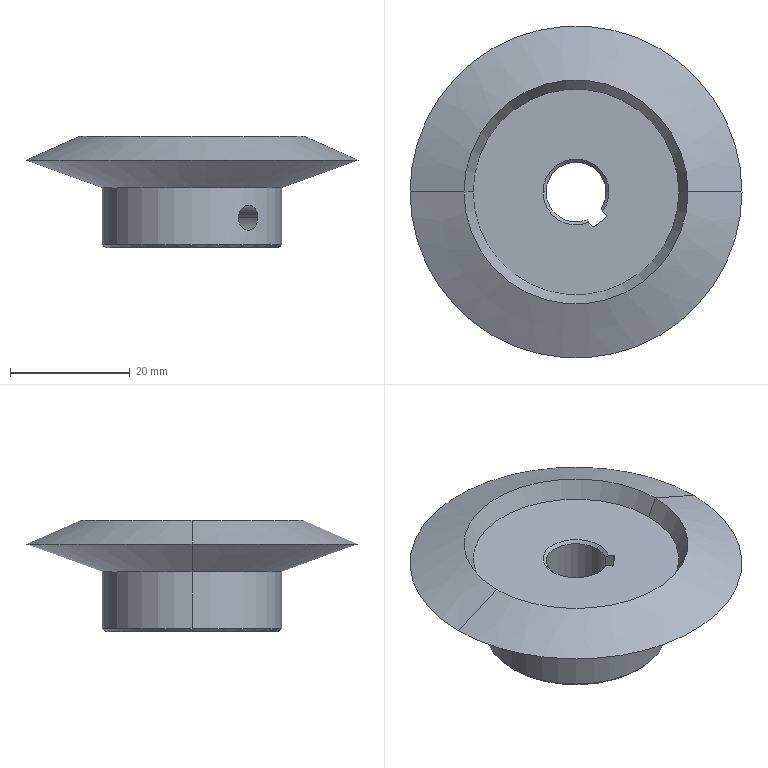Part | SolidWorks | features BaseBody 1 | 1 solid | 33 faces | box 55.34 x 55.34 x 18.54 mm | volume 16079 mm3 | cone 14 | cylinder 11 | plane 8 | commonest cylinder face diameters 0.4 x4 10 x3 4.2 x2 30 x2
STEP:
#1=CARTESIAN_POINT('',(-119.453,1729.544,-1197.43));
#2=VERTEX_POINT('',#1);
#3=CARTESIAN_POINT('',(-149.453,1729.544,-1197.43));
#4=VERTEX_POINT('',#3);
#5=CARTESIAN_POINT('',(-134.453,1729.544,-1197.43));
#6=DIRECTION('',(0.,0.,1.));
#7=DIRECTION('',(-0.7769,-0.6296,0.));
#8=AXIS2_PLACEMENT_3D('',#5,#6,#7);
#9=CIRCLE('',#8,15.);
#10=EDGE_CURVE('',#2,#4,#9,.T.);
#11=ORIENTED_EDGE('',*,*,#10,.T.);
#12=CARTESIAN_POINT('',(-162.123,1729.544,-1192.84));
#13=VERTEX_POINT('',#12);
#14=CARTESIAN_POINT('',(-162.123,1729.544,-1192.84));
#15=DIRECTION('',(-0.9402,0.,0.3406));
#16=VECTOR('',#15,1000.);
#17=LINE('',#14,#16);
#18=EDGE_CURVE('',#4,#13,#17,.T.);
#19=ORIENTED_EDGE('',*,*,#18,.T.);
#20=CARTESIAN_POINT('',(-106.783,1729.544,-1192.84));
#21=VERTEX_POINT('',#20);
#22=CARTESIAN_POINT('',(-134.453,1729.544,-1192.84));
#23=DIRECTION('',(0.,0.,-1.));
#24=DIRECTION('',(-0.7769,-0.6296,0.));
#25=AXIS2_PLACEMENT_3D('',#22,#23,#24);
#26=CIRCLE('',#25,27.67);
#27=EDGE_CURVE('',#13,#21,#26,.T.);
#28=ORIENTED_EDGE('',*,*,#27,.T.);
#29=CARTESIAN_POINT('',(-106.783,1729.544,-1192.84));
#30=DIRECTION('',(0.9402,0.,0.3406));
#31=VECTOR('',#30,1000.);
#32=LINE('',#29,#31);
#33=EDGE_CURVE('',#2,#21,#32,.T.);
#34=ORIENTED_EDGE('',*,*,#33,.F.);
#35=EDGE_LOOP('',(#11,#19,#28,#34));
#36=FACE_OUTER_BOUND('',#35,.T.);
#37=CARTESIAN_POINT('',(-134.453,1729.544,-1192.84));
#38=DIRECTION('',(0.,0.,1.));
#39=DIRECTION('',(1.,0.,0.));
#40=AXIS2_PLACEMENT_3D('',#37,#38,#39);
#41=CONICAL_SURFACE('',#40,27.67,1.223);
#42=ADVANCED_FACE('',(#36),#41,.T.);
#43=CARTESIAN_POINT('',(-153.134,1729.544,-1188.89));
#44=VERTEX_POINT('',#43);
#45=CARTESIAN_POINT('',(-115.773,1729.544,-1188.89));
#46=VERTEX_POINT('',#45);
#47=CARTESIAN_POINT('',(-134.453,1729.544,-1188.89));
#48=DIRECTION('',(0.,0.,-1.));
#49=DIRECTION('',(0.7769,0.6296,0.));
#50=AXIS2_PLACEMENT_3D('',#47,#48,#49);
#51=CIRCLE('',#50,18.68);
#52=EDGE_CURVE('',#44,#46,#51,.T.);
#53=ORIENTED_EDGE('',*,*,#52,.T.);
#54=CARTESIAN_POINT('',(-106.783,1729.544,-1192.84));
#55=DIRECTION('',(0.9155,0.,-0.4023));
#56=VECTOR('',#55,1000.);
#57=LINE('',#54,#56);
#58=EDGE_CURVE('',#46,#21,#57,.T.);
#59=ORIENTED_EDGE('',*,*,#58,.T.);
#60=ORIENTED_EDGE('',*,*,#27,.F.);
#61=CARTESIAN_POINT('',(-162.123,1729.544,-1192.84));
#62=DIRECTION('',(-0.9155,0.,-0.4023));
#63=VECTOR('',#62,1000.);
#64=LINE('',#61,#63);
#65=EDGE_CURVE('',#44,#13,#64,.T.);
#66=ORIENTED_EDGE('',*,*,#65,.F.);
#67=EDGE_LOOP('',(#53,#59,#60,#66));
#68=FACE_OUTER_BOUND('',#67,.T.);
#69=CARTESIAN_POINT('',(-134.453,1729.544,-1192.84));
#70=DIRECTION('',(0.,0.,-1.));
#71=DIRECTION('',(-1.,0.,0.));
#72=AXIS2_PLACEMENT_3D('',#69,#70,#71);
#73=CONICAL_SURFACE('',#72,27.67,1.157);
#74=ADVANCED_FACE('',(#68),#73,.T.);
#75=CARTESIAN_POINT('',(-119.453,1729.544,-1206.93));
#76=VERTEX_POINT('',#75);
#77=CARTESIAN_POINT('',(-149.453,1729.544,-1206.93));
#78=VERTEX_POINT('',#77);
#79=CARTESIAN_POINT('',(-134.453,1729.544,-1206.93));
#80=DIRECTION('',(0.,0.,1.));
#81=DIRECTION('',(1.,0.,0.));
#82=AXIS2_PLACEMENT_3D('',#79,#80,#81);
#83=CIRCLE('',#82,15.);
#84=EDGE_CURVE('',#76,#78,#83,.T.);
#85=ORIENTED_EDGE('',*,*,#84,.T.);
#86=CARTESIAN_POINT('',(-149.453,1729.544,-1180.68));
#87=DIRECTION('',(0.,0.,1.));
#88=VECTOR('',#87,1000.);
#89=LINE('',#86,#88);
#90=EDGE_CURVE('',#78,#4,#89,.T.);
#91=ORIENTED_EDGE('',*,*,#90,.T.);
#92=ORIENTED_EDGE('',*,*,#10,.F.);
#93=CARTESIAN_POINT('',(-119.453,1729.544,-1180.68));
#94=DIRECTION('',(0.,0.,1.));
#95=VECTOR('',#94,1000.);
#96=LINE('',#93,#95);
#97=EDGE_CURVE('',#76,#2,#96,.T.);
#98=ORIENTED_EDGE('',*,*,#97,.F.);
#99=EDGE_LOOP('',(#85,#91,#92,#98));
#100=FACE_OUTER_BOUND('',#99,.T.);
#101=CARTESIAN_POINT('',(-134.453,1729.544,-1180.68));
#102=DIRECTION('',(0.,0.,1.));
#103=DIRECTION('',(1.,0.,0.));
#104=AXIS2_PLACEMENT_3D('',#101,#102,#103);
#105=CYLINDRICAL_SURFACE('',#104,15.);
#106=ADVANCED_FACE('',(#100),#105,.T.);
#107=CARTESIAN_POINT('',(-151.603,1729.544,-1191.93));
#108=VERTEX_POINT('',#107);
#109=CARTESIAN_POINT('',(-117.303,1729.544,-1191.93));
#110=VERTEX_POINT('',#109);
#111=CARTESIAN_POINT('',(-134.453,1729.544,-1191.93));
#112=DIRECTION('',(0.,0.,1.));
#113=DIRECTION('',(1.,0.,0.));
#114=AXIS2_PLACEMENT_3D('',#111,#112,#113);
#115=CIRCLE('',#114,17.15);
#116=EDGE_CURVE('',#108,#110,#115,.T.);
#117=ORIENTED_EDGE('',*,*,#116,.F.);
#118=CARTESIAN_POINT('',(-153.134,1729.544,-1188.89));
#119=DIRECTION('',(-0.4496,0.,0.8932));
#120=VECTOR('',#119,1000.);
#121=LINE('',#118,#120);
#122=EDGE_CURVE('',#108,#44,#121,.T.);
#123=ORIENTED_EDGE('',*,*,#122,.T.);
#124=CARTESIAN_POINT('',(-134.453,1729.544,-1188.89));
#125=DIRECTION('',(0.,0.,-1.));
#126=DIRECTION('',(0.7769,0.6296,0.));
#127=AXIS2_PLACEMENT_3D('',#124,#125,#126);
#128=CIRCLE('',#127,18.68);
#129=EDGE_CURVE('',#46,#44,#128,.T.);
#130=ORIENTED_EDGE('',*,*,#129,.F.);
#131=CARTESIAN_POINT('',(-115.773,1729.544,-1188.89));
#132=DIRECTION('',(0.4496,0.,0.8932));
#133=VECTOR('',#132,1000.);
#134=LINE('',#131,#133);
#135=EDGE_CURVE('',#110,#46,#134,.T.);
#136=ORIENTED_EDGE('',*,*,#135,.F.);
#137=EDGE_LOOP('',(#117,#123,#130,#136));
#138=FACE_OUTER_BOUND('',#137,.T.);
#139=CARTESIAN_POINT('',(-134.453,1729.544,-1188.89));
#140=DIRECTION('',(0.,0.,1.));
#141=DIRECTION('',(1.,0.,0.));
#142=AXIS2_PLACEMENT_3D('',#139,#140,#141);
#143=CONICAL_SURFACE('',#142,18.68,0.4663);
#144=ADVANCED_FACE('',(#138),#143,.F.);
#145=CARTESIAN_POINT('',(-133.228,1724.696,-1202.43));
#146=VERTEX_POINT('',#145);
#147=CARTESIAN_POINT('',(-132.616,1724.894,-1203.9));
#148=VERTEX_POINT('',#147);
#149=CARTESIAN_POINT('',(-133.228,1724.696,-1202.43));
#150=CARTESIAN_POINT('',(-133.228,1724.696,-1202.569));
#151=CARTESIAN_POINT('',(-133.214,1724.7,-1202.704));
#152=CARTESIAN_POINT('',(-133.158,1724.715,-1202.971));
#153=CARTESIAN_POINT('',(-133.115,1724.726,-1203.104));
#154=CARTESIAN_POINT('',(-132.954,1724.773,-1203.479));
#155=CARTESIAN_POINT('',(-132.8,1724.821,-1203.707));
#156=CARTESIAN_POINT('',(-132.616,1724.894,-1203.9));
#157=B_SPLINE_CURVE_WITH_KNOTS('',3,(#149,#150,#151,#152,#153,#154,#155,#156),.UNSPECIFIED.,.F.,.F.,(4,2,2,4),(0.001639,0.002049,0.002458,0.003277),.UNSPECIFIED.);
#158=EDGE_CURVE('',#146,#148,#157,.T.);
#159=ORIENTED_EDGE('',*,*,#158,.F.);
#160=CARTESIAN_POINT('',(-126.734,1716.683,-1202.43));
#161=VERTEX_POINT('',#160);
#162=CARTESIAN_POINT('',(-126.641,1716.568,-1202.43));
#163=DIRECTION('',(0.6296,-0.7769,0.));
#164=VECTOR('',#163,1000.);
#165=LINE('',#162,#164);
#166=EDGE_CURVE('',#146,#161,#165,.T.);
#167=ORIENTED_EDGE('',*,*,#166,.T.);
#168=CARTESIAN_POINT('',(-123.471,1719.327,-1202.43));
#169=VERTEX_POINT('',#168);
#170=CARTESIAN_POINT('',(-123.471,1719.327,-1202.43));
#171=CARTESIAN_POINT('',(-123.471,1719.327,-1202.569));
#172=CARTESIAN_POINT('',(-123.48,1719.317,-1202.705));
#173=CARTESIAN_POINT('',(-123.517,1719.278,-1202.974));
#174=CARTESIAN_POINT('',(-123.545,1719.248,-1203.107));
#175=CARTESIAN_POINT('',(-123.618,1719.171,-1203.362));
#176=CARTESIAN_POINT('',(-123.663,1719.124,-1203.482));
#177=CARTESIAN_POINT('',(-123.771,1719.014,-1203.71));
#178=CARTESIAN_POINT('',(-123.833,1718.951,-1203.818));
#179=CARTESIAN_POINT('',(-124.04,1718.746,-1204.108));
#180=CARTESIAN_POINT('',(-124.21,1718.583,-1204.265));
#181=CARTESIAN_POINT('',(-124.586,1718.244,-1204.474));
#182=CARTESIAN_POINT('',(-124.795,1718.064,-1204.53));
#183=CARTESIAN_POINT('',(-125.115,1717.805,-1204.53));
#184=CARTESIAN_POINT('',(-125.224,1717.719,-1204.516));
#185=CARTESIAN_POINT('',(-125.438,1717.555,-1204.463));
#186=CARTESIAN_POINT('',(-125.543,1717.476,-1204.423));
#187=CARTESIAN_POINT('',(-125.75,1717.327,-1204.318));
#188=CARTESIAN_POINT('',(-125.85,1717.256,-1204.252));
#189=CARTESIAN_POINT('',(-126.038,1717.126,-1204.101));
#190=CARTESIAN_POINT('',(-126.127,1717.067,-1204.014));
#191=CARTESIAN_POINT('',(-126.291,1716.959,-1203.818));
#192=CARTESIAN_POINT('',(-126.365,1716.912,-1203.712));
#193=CARTESIAN_POINT('',(-126.494,1716.83,-1203.485));
#194=CARTESIAN_POINT('',(-126.55,1716.795,-1203.362));
#195=CARTESIAN_POINT('',(-126.641,1716.739,-1203.108));
#196=CARTESIAN_POINT('',(-126.675,1716.718,-1202.977));
#197=CARTESIAN_POINT('',(-126.722,1716.69,-1202.708));
#198=CARTESIAN_POINT('',(-126.734,1716.683,-1202.569));
#199=CARTESIAN_POINT('',(-126.734,1716.683,-1202.43));
#200=B_SPLINE_CURVE_WITH_KNOTS('',3,(#170,#171,#172,#173,#174,#175,#176,#177,#178,#179,#180,#181,#182,#183,#184,#185,#186,#187,#188,#189,#190,#191,#192,#193,#194,#195,#196,#197,#198,#199),.UNSPECIFIED.,.F.,.F.,(4,2,2,2,2,2,2,2,2,2,2,2,2,2,4),(0.006572,0.006983,0.007394,0.007804,0.008215,0.009037,0.009858,0.01027,0.01068,0.01109,0.0115,0.01191,0.01232,0.01273,0.01314),.UNSPECIFIED.);
#201=EDGE_CURVE('',#169,#161,#200,.T.);
#202=ORIENTED_EDGE('',*,*,#201,.F.);
#203=CARTESIAN_POINT('',(-129.965,1727.341,-1202.43));
#204=VERTEX_POINT('',#203);
#205=CARTESIAN_POINT('',(-123.378,1719.212,-1202.43));
#206=DIRECTION('',(0.6296,-0.7769,0.));
#207=VECTOR('',#206,1000.);
#208=LINE('',#205,#207);
#209=EDGE_CURVE('',#204,#169,#208,.T.);
#210=ORIENTED_EDGE('',*,*,#209,.F.);
#211=CARTESIAN_POINT('',(-130.285,1726.783,-1203.9));
#212=VERTEX_POINT('',#211);
#213=CARTESIAN_POINT('',(-130.285,1726.783,-1203.9));
#214=CARTESIAN_POINT('',(-130.23,1726.865,-1203.803));
#215=CARTESIAN_POINT('',(-130.184,1726.941,-1203.699));
#216=CARTESIAN_POINT('',(-130.104,1727.077,-1203.476));
#217=CARTESIAN_POINT('',(-130.07,1727.137,-1203.355));
#218=CARTESIAN_POINT('',(-130.018,1727.236,-1203.104));
#219=CARTESIAN_POINT('',(-129.998,1727.275,-1202.975));
#220=CARTESIAN_POINT('',(-129.972,1727.327,-1202.707));
#221=CARTESIAN_POINT('',(-129.965,1727.341,-1202.569));
#222=CARTESIAN_POINT('',(-129.965,1727.341,-1202.43));
#223=B_SPLINE_CURVE_WITH_KNOTS('',3,(#213,#214,#215,#216,#217,#218,#219,#220,#221,#222),.UNSPECIFIED.,.F.,.F.,(4,2,2,2,4),(-0.001639,-0.001229,-0.0008193,-0.0004097,0.),.UNSPECIFIED.);
#224=EDGE_CURVE('',#212,#204,#223,.T.);
#225=ORIENTED_EDGE('',*,*,#224,.F.);
#226=CARTESIAN_POINT('',(-129.385,1725.671,-1203.9));
#227=VERTEX_POINT('',#226);
#228=CARTESIAN_POINT('',(-123.844,1718.835,-1203.9));
#229=DIRECTION('',(-0.6296,0.7769,0.));
#230=VECTOR('',#229,1000.);
#231=LINE('',#228,#230);
#232=EDGE_CURVE('',#227,#212,#231,.T.);
#233=ORIENTED_EDGE('',*,*,#232,.F.);
#234=CARTESIAN_POINT('',(-129.414,1725.39,-1204.079));
#235=VERTEX_POINT('',#234);
#236=CARTESIAN_POINT('',(-129.414,1725.39,-1204.079));
#237=CARTESIAN_POINT('',(-129.376,1725.421,-1204.041));
#238=CARTESIAN_POINT('',(-129.351,1725.463,-1204.001));
#239=CARTESIAN_POINT('',(-129.334,1725.562,-1203.931));
#240=CARTESIAN_POINT('',(-129.345,1725.623,-1203.9));
#241=CARTESIAN_POINT('',(-129.385,1725.671,-1203.9));
#242=B_SPLINE_CURVE_WITH_KNOTS('',3,(#236,#237,#238,#239,#240,#241),.UNSPECIFIED.,.F.,.F.,(4,2,4),(0.,0.0001833,0.0003667),.UNSPECIFIED.);
#243=EDGE_CURVE('',#235,#227,#242,.T.);
#244=ORIENTED_EDGE('',*,*,#243,.F.);
#245=CARTESIAN_POINT('',(-131.434,1723.753,-1204.079));
#246=VERTEX_POINT('',#245);
#247=CARTESIAN_POINT('',(-130.424,1724.572,-1202.43));
#248=DIRECTION('',(0.6296,-0.7769,0.));
#249=DIRECTION('',(0.7769,0.6296,0.));
#250=AXIS2_PLACEMENT_3D('',#247,#248,#249);
#251=CIRCLE('',#250,2.1);
#252=EDGE_CURVE('',#246,#235,#251,.T.);
#253=ORIENTED_EDGE('',*,*,#252,.F.);
#254=CARTESIAN_POINT('',(-131.715,1723.783,-1203.9));
#255=VERTEX_POINT('',#254);
#256=CARTESIAN_POINT('',(-131.715,1723.783,-1203.9));
#257=CARTESIAN_POINT('',(-131.676,1723.734,-1203.9));
#258=CARTESIAN_POINT('',(-131.619,1723.711,-1203.93));
#259=CARTESIAN_POINT('',(-131.518,1723.707,-1204.001));
#260=CARTESIAN_POINT('',(-131.472,1723.723,-1204.041));
#261=CARTESIAN_POINT('',(-131.434,1723.753,-1204.079));
#262=B_SPLINE_CURVE_WITH_KNOTS('',3,(#256,#257,#258,#259,#260,#261),.UNSPECIFIED.,.F.,.F.,(4,2,4),(0.,0.0001836,0.0003672),.UNSPECIFIED.);
#263=EDGE_CURVE('',#255,#246,#262,.T.);
#264=ORIENTED_EDGE('',*,*,#263,.F.);
#265=CARTESIAN_POINT('',(-126.175,1716.946,-1203.9));
#266=DIRECTION('',(0.6296,-0.7769,0.));
#267=VECTOR('',#266,1000.);
#268=LINE('',#265,#267);
#269=EDGE_CURVE('',#148,#255,#268,.T.);
#270=ORIENTED_EDGE('',*,*,#269,.F.);
#271=EDGE_LOOP('',(#159,#167,#202,#210,#225,#233,#244,#253,#264,#270));
#272=FACE_OUTER_BOUND('',#271,.T.);
#273=CARTESIAN_POINT('',(-125.01,1717.89,-1202.43));
#274=DIRECTION('',(0.6296,-0.7769,0.));
#275=DIRECTION('',(0.7769,0.6296,0.));
#276=AXIS2_PLACEMENT_3D('',#273,#274,#275);
#277=CYLINDRICAL_SURFACE('',#276,2.1);
#278=ADVANCED_FACE('',(#272),#277,.F.);
#279=CARTESIAN_POINT('',(-119.953,1729.544,-1207.43));
#280=VERTEX_POINT('',#279);
#281=CARTESIAN_POINT('',(-148.953,1729.544,-1207.43));
#282=VERTEX_POINT('',#281);
#283=CARTESIAN_POINT('',(-134.453,1729.544,-1207.43));
#284=DIRECTION('',(0.,0.,1.));
#285=DIRECTION('',(1.,0.,0.));
#286=AXIS2_PLACEMENT_3D('',#283,#284,#285);
#287=CIRCLE('',#286,14.5);
#288=EDGE_CURVE('',#280,#282,#287,.T.);
#289=ORIENTED_EDGE('',*,*,#288,.T.);
#290=CARTESIAN_POINT('',(-149.453,1729.544,-1206.93));
#291=DIRECTION('',(-0.7071,0.,0.7071));
#292=VECTOR('',#291,1000.);
#293=LINE('',#290,#292);
#294=EDGE_CURVE('',#282,#78,#293,.T.);
#295=ORIENTED_EDGE('',*,*,#294,.T.);
#296=ORIENTED_EDGE('',*,*,#84,.F.);
#297=CARTESIAN_POINT('',(-119.453,1729.544,-1206.93));
#298=DIRECTION('',(0.7071,0.,0.7071));
#299=VECTOR('',#298,1000.);
#300=LINE('',#297,#299);
#301=EDGE_CURVE('',#280,#76,#300,.T.);
#302=ORIENTED_EDGE('',*,*,#301,.F.);
#303=EDGE_LOOP('',(#289,#295,#296,#302));
#304=FACE_OUTER_BOUND('',#303,.T.);
#305=CARTESIAN_POINT('',(-134.453,1729.544,-1206.93));
#306=DIRECTION('',(0.,0.,1.));
#307=DIRECTION('',(1.,0.,0.));
#308=AXIS2_PLACEMENT_3D('',#305,#306,#307);
#309=CONICAL_SURFACE('',#308,15.,0.7854);
#310=ADVANCED_FACE('',(#304),#309,.T.);
#311=CARTESIAN_POINT('',(-139.453,1729.544,-1206.93));
#312=VERTEX_POINT('',#311);
#313=CARTESIAN_POINT('',(-132.616,1724.894,-1206.93));
#314=VERTEX_POINT('',#313);
#315=CARTESIAN_POINT('',(-134.453,1729.544,-1206.93));
#316=DIRECTION('',(0.,0.,1.));
#317=DIRECTION('',(1.,0.,0.));
#318=AXIS2_PLACEMENT_3D('',#315,#316,#317);
#319=CIRCLE('',#318,5.);
#320=EDGE_CURVE('',#312,#314,#319,.T.);
#321=ORIENTED_EDGE('',*,*,#320,.F.);
#322=CARTESIAN_POINT('',(-139.453,1729.544,-1192.43));
#323=VERTEX_POINT('',#322);
#324=CARTESIAN_POINT('',(-139.453,1729.544,-1180.68));
#325=DIRECTION('',(0.,0.,1.));
#326=VECTOR('',#325,1000.);
#327=LINE('',#324,#326);
#328=EDGE_CURVE('',#312,#323,#327,.T.);
#329=ORIENTED_EDGE('',*,*,#328,.T.);
#330=CARTESIAN_POINT('',(-132.616,1724.894,-1192.43));
#331=VERTEX_POINT('',#330);
#332=CARTESIAN_POINT('',(-134.453,1729.544,-1192.43));
#333=DIRECTION('',(0.,0.,-1.));
#334=DIRECTION('',(1.,0.,0.));
#335=AXIS2_PLACEMENT_3D('',#332,#333,#334);
#336=CIRCLE('',#335,5.);
#337=EDGE_CURVE('',#331,#323,#336,.T.);
#338=ORIENTED_EDGE('',*,*,#337,.F.);
#339=CARTESIAN_POINT('',(-132.616,1724.894,-1200.96));
#340=VERTEX_POINT('',#339);
#341=CARTESIAN_POINT('',(-132.616,1724.894,-1188.89));
#342=DIRECTION('',(0.,0.,-1.));
#343=VECTOR('',#342,1000.);
#344=LINE('',#341,#343);
#345=EDGE_CURVE('',#331,#340,#344,.T.);
#346=ORIENTED_EDGE('',*,*,#345,.T.);
#347=CARTESIAN_POINT('',(-132.616,1724.894,-1200.96));
#348=CARTESIAN_POINT('',(-132.708,1724.857,-1201.057));
#349=CARTESIAN_POINT('',(-132.792,1724.828,-1201.161));
#350=CARTESIAN_POINT('',(-132.941,1724.778,-1201.384));
#351=CARTESIAN_POINT('',(-133.007,1724.757,-1201.505));
#352=CARTESIAN_POINT('',(-133.115,1724.726,-1201.756));
#353=CARTESIAN_POINT('',(-133.157,1724.715,-1201.885));
#354=CARTESIAN_POINT('',(-133.213,1724.7,-1202.153));
#355=CARTESIAN_POINT('',(-133.228,1724.696,-1202.291));
#356=CARTESIAN_POINT('',(-133.228,1724.696,-1202.43));
#357=B_SPLINE_CURVE_WITH_KNOTS('',3,(#347,#348,#349,#350,#351,#352,#353,#354,#355,#356),.UNSPECIFIED.,.F.,.F.,(4,2,2,2,4),(0.,0.0004098,0.0008196,0.001229,0.001639),.UNSPECIFIED.);
#358=EDGE_CURVE('',#340,#146,#357,.T.);
#359=ORIENTED_EDGE('',*,*,#358,.T.);
#360=ORIENTED_EDGE('',*,*,#158,.T.);
#361=CARTESIAN_POINT('',(-132.616,1724.894,-1180.68));
#362=DIRECTION('',(0.,0.,1.));
#363=VECTOR('',#362,1000.);
#364=LINE('',#361,#363);
#365=EDGE_CURVE('',#314,#148,#364,.T.);
#366=ORIENTED_EDGE('',*,*,#365,.F.);
#367=EDGE_LOOP('',(#321,#329,#338,#346,#359,#360,#366));
#368=FACE_OUTER_BOUND('',#367,.T.);
#369=CARTESIAN_POINT('',(-134.453,1729.544,-1180.68));
#370=DIRECTION('',(0.,0.,1.));
#371=DIRECTION('',(1.,0.,0.));
#372=AXIS2_PLACEMENT_3D('',#369,#370,#371);
#373=CYLINDRICAL_SURFACE('',#372,5.);
#374=ADVANCED_FACE('',(#368),#373,.F.);
#375=ORIENTED_EDGE('',*,*,#328,.F.);
#376=CARTESIAN_POINT('',(-129.453,1729.544,-1206.93));
#377=VERTEX_POINT('',#376);
#378=CARTESIAN_POINT('',(-134.453,1729.544,-1206.93));
#379=DIRECTION('',(0.,0.,1.));
#380=DIRECTION('',(1.,0.,0.));
#381=AXIS2_PLACEMENT_3D('',#378,#379,#380);
#382=CIRCLE('',#381,5.);
#383=EDGE_CURVE('',#377,#312,#382,.T.);
#384=ORIENTED_EDGE('',*,*,#383,.F.);
#385=CARTESIAN_POINT('',(-129.453,1729.544,-1192.43));
#386=VERTEX_POINT('',#385);
#387=CARTESIAN_POINT('',(-129.453,1729.544,-1180.68));
#388=DIRECTION('',(0.,0.,1.));
#389=VECTOR('',#388,1000.);
#390=LINE('',#387,#389);
#391=EDGE_CURVE('',#377,#386,#390,.T.);
#392=ORIENTED_EDGE('',*,*,#391,.T.);
#393=CARTESIAN_POINT('',(-134.453,1729.544,-1192.43));
#394=DIRECTION('',(0.,0.,-1.));
#395=DIRECTION('',(1.,0.,0.));
#396=AXIS2_PLACEMENT_3D('',#393,#394,#395);
#397=CIRCLE('',#396,5.);
#398=EDGE_CURVE('',#323,#386,#397,.T.);
#399=ORIENTED_EDGE('',*,*,#398,.F.);
#400=EDGE_LOOP('',(#375,#384,#392,#399));
#401=FACE_OUTER_BOUND('',#400,.T.);
#402=CARTESIAN_POINT('',(-134.453,1729.544,-1180.68));
#403=DIRECTION('',(0.,0.,1.));
#404=DIRECTION('',(1.,0.,0.));
#405=AXIS2_PLACEMENT_3D('',#402,#403,#404);
#406=CYLINDRICAL_SURFACE('',#405,5.);
#407=ADVANCED_FACE('',(#401),#406,.F.);
#408=ORIENTED_EDGE('',*,*,#337,.T.);
#409=CARTESIAN_POINT('',(-139.953,1729.544,-1191.93));
#410=VERTEX_POINT('',#409);
#411=CARTESIAN_POINT('',(-139.953,1729.544,-1191.93));
#412=DIRECTION('',(-0.7071,0.,0.7071));
#413=VECTOR('',#412,1000.);
#414=LINE('',#411,#413);
#415=EDGE_CURVE('',#323,#410,#414,.T.);
#416=ORIENTED_EDGE('',*,*,#415,.T.);
#417=CARTESIAN_POINT('',(-132.287,1724.489,-1191.93));
#418=VERTEX_POINT('',#417);
#419=CARTESIAN_POINT('',(-134.453,1729.544,-1191.93));
#420=DIRECTION('',(0.,0.,1.));
#421=DIRECTION('',(1.,0.,0.));
#422=AXIS2_PLACEMENT_3D('',#419,#420,#421);
#423=CIRCLE('',#422,5.5);
#424=EDGE_CURVE('',#410,#418,#423,.T.);
#425=ORIENTED_EDGE('',*,*,#424,.T.);
#426=CARTESIAN_POINT('',(-132.287,1724.489,-1191.93));
#427=CARTESIAN_POINT('',(-132.397,1724.623,-1192.097));
#428=CARTESIAN_POINT('',(-132.506,1724.758,-1192.264));
#429=CARTESIAN_POINT('',(-132.616,1724.894,-1192.43));
#430=B_SPLINE_CURVE_WITH_KNOTS('',3,(#426,#427,#428,#429),.UNSPECIFIED.,.F.,.F.,(4,4),(0.,0.0007227),.UNSPECIFIED.);
#431=EDGE_CURVE('',#418,#331,#430,.T.);
#432=ORIENTED_EDGE('',*,*,#431,.T.);
#433=EDGE_LOOP('',(#408,#416,#425,#432));
#434=FACE_OUTER_BOUND('',#433,.T.);
#435=CARTESIAN_POINT('',(-134.453,1729.544,-1191.93));
#436=DIRECTION('',(0.,0.,1.));
#437=DIRECTION('',(1.,0.,0.));
#438=AXIS2_PLACEMENT_3D('',#435,#436,#437);
#439=CONICAL_SURFACE('',#438,5.5,0.7854);
#440=ADVANCED_FACE('',(#434),#439,.F.);
#441=ORIENTED_EDGE('',*,*,#415,.F.);
#442=ORIENTED_EDGE('',*,*,#398,.T.);
#443=CARTESIAN_POINT('',(-128.953,1729.544,-1191.93));
#444=VERTEX_POINT('',#443);
#445=CARTESIAN_POINT('',(-128.953,1729.544,-1191.93));
#446=DIRECTION('',(0.7071,0.,0.7071));
#447=VECTOR('',#446,1000.);
#448=LINE('',#445,#447);
#449=EDGE_CURVE('',#386,#444,#448,.T.);
#450=ORIENTED_EDGE('',*,*,#449,.T.);
#451=CARTESIAN_POINT('',(-134.453,1729.544,-1191.93));
#452=DIRECTION('',(0.,0.,1.));
#453=DIRECTION('',(1.,0.,0.));
#454=AXIS2_PLACEMENT_3D('',#451,#452,#453);
#455=CIRCLE('',#454,5.5);
#456=EDGE_CURVE('',#444,#410,#455,.T.);
#457=ORIENTED_EDGE('',*,*,#456,.T.);
#458=EDGE_LOOP('',(#441,#442,#450,#457));
#459=FACE_OUTER_BOUND('',#458,.T.);
#460=CARTESIAN_POINT('',(-134.453,1729.544,-1191.93));
#461=DIRECTION('',(0.,0.,1.));
#462=DIRECTION('',(1.,0.,0.));
#463=AXIS2_PLACEMENT_3D('',#460,#461,#462);
#464=CONICAL_SURFACE('',#463,5.5,0.7854);
#465=ADVANCED_FACE('',(#459),#464,.F.);
#466=CARTESIAN_POINT('',(-130.285,1726.783,-1206.93));
#467=VERTEX_POINT('',#466);
#468=CARTESIAN_POINT('',(-134.453,1729.544,-1206.93));
#469=DIRECTION('',(0.,0.,1.));
#470=DIRECTION('',(1.,0.,0.));
#471=AXIS2_PLACEMENT_3D('',#468,#469,#470);
#472=CIRCLE('',#471,5.);
#473=EDGE_CURVE('',#467,#377,#472,.T.);
#474=ORIENTED_EDGE('',*,*,#473,.T.);
#475=CARTESIAN_POINT('',(-128.953,1729.544,-1207.43));
#476=VERTEX_POINT('',#475);
#477=CARTESIAN_POINT('',(-128.953,1729.544,-1207.43));
#478=DIRECTION('',(0.7071,0.,-0.7071));
#479=VECTOR('',#478,1000.);
#480=LINE('',#477,#479);
#481=EDGE_CURVE('',#377,#476,#480,.T.);
#482=ORIENTED_EDGE('',*,*,#481,.T.);
#483=CARTESIAN_POINT('',(-129.957,1726.377,-1207.43));
#484=VERTEX_POINT('',#483);
#485=CARTESIAN_POINT('',(-134.453,1729.544,-1207.43));
#486=DIRECTION('',(0.,0.,-1.));
#487=DIRECTION('',(-1.,0.,0.));
#488=AXIS2_PLACEMENT_3D('',#485,#486,#487);
#489=CIRCLE('',#488,5.5);
#490=EDGE_CURVE('',#476,#484,#489,.T.);
#491=ORIENTED_EDGE('',*,*,#490,.T.);
#492=CARTESIAN_POINT('',(-129.957,1726.377,-1207.43));
#493=CARTESIAN_POINT('',(-130.066,1726.512,-1207.263));
#494=CARTESIAN_POINT('',(-130.175,1726.647,-1207.096));
#495=CARTESIAN_POINT('',(-130.285,1726.783,-1206.93));
#496=B_SPLINE_CURVE_WITH_KNOTS('',3,(#492,#493,#494,#495),.UNSPECIFIED.,.F.,.F.,(4,4),(0.,0.0007227),.UNSPECIFIED.);
#497=EDGE_CURVE('',#484,#467,#496,.T.);
#498=ORIENTED_EDGE('',*,*,#497,.T.);
#499=EDGE_LOOP('',(#474,#482,#491,#498));
#500=FACE_OUTER_BOUND('',#499,.T.);
#501=CARTESIAN_POINT('',(-134.453,1729.544,-1207.43));
#502=DIRECTION('',(0.,0.,-1.));
#503=DIRECTION('',(-1.,0.,0.));
#504=AXIS2_PLACEMENT_3D('',#501,#502,#503);
#505=CONICAL_SURFACE('',#504,5.5,0.7854);
#506=ADVANCED_FACE('',(#500),#505,.F.);
#507=ORIENTED_EDGE('',*,*,#481,.F.);
#508=ORIENTED_EDGE('',*,*,#383,.T.);
#509=CARTESIAN_POINT('',(-139.953,1729.544,-1207.43));
#510=VERTEX_POINT('',#509);
#511=CARTESIAN_POINT('',(-139.953,1729.544,-1207.43));
#512=DIRECTION('',(-0.7071,0.,-0.7071));
#513=VECTOR('',#512,1000.);
#514=LINE('',#511,#513);
#515=EDGE_CURVE('',#312,#510,#514,.T.);
#516=ORIENTED_EDGE('',*,*,#515,.T.);
#517=CARTESIAN_POINT('',(-134.453,1729.544,-1207.43));
#518=DIRECTION('',(0.,0.,-1.));
#519=DIRECTION('',(-1.,0.,0.));
#520=AXIS2_PLACEMENT_3D('',#517,#518,#519);
#521=CIRCLE('',#520,5.5);
#522=EDGE_CURVE('',#510,#476,#521,.T.);
#523=ORIENTED_EDGE('',*,*,#522,.T.);
#524=EDGE_LOOP('',(#507,#508,#516,#523));
#525=FACE_OUTER_BOUND('',#524,.T.);
#526=CARTESIAN_POINT('',(-134.453,1729.544,-1207.43));
#527=DIRECTION('',(0.,0.,-1.));
#528=DIRECTION('',(-1.,0.,0.));
#529=AXIS2_PLACEMENT_3D('',#526,#527,#528);
#530=CONICAL_SURFACE('',#529,5.5,0.7854);
#531=ADVANCED_FACE('',(#525),#530,.F.);
#532=ORIENTED_EDGE('',*,*,#18,.F.);
#533=CARTESIAN_POINT('',(-134.453,1729.544,-1197.43));
#534=DIRECTION('',(0.,0.,1.));
#535=DIRECTION('',(-0.7769,-0.6296,0.));
#536=AXIS2_PLACEMENT_3D('',#533,#534,#535);
#537=CIRCLE('',#536,15.);
#538=EDGE_CURVE('',#4,#2,#537,.T.);
#539=ORIENTED_EDGE('',*,*,#538,.T.);
#540=ORIENTED_EDGE('',*,*,#33,.T.);
#541=CARTESIAN_POINT('',(-134.453,1729.544,-1192.84));
#542=DIRECTION('',(0.,0.,-1.));
#543=DIRECTION('',(-0.7769,-0.6296,0.));
#544=AXIS2_PLACEMENT_3D('',#541,#542,#543);
#545=CIRCLE('',#544,27.67);
#546=EDGE_CURVE('',#21,#13,#545,.T.);
#547=ORIENTED_EDGE('',*,*,#546,.T.);
#548=EDGE_LOOP('',(#532,#539,#540,#547));
#549=FACE_OUTER_BOUND('',#548,.T.);
#550=CARTESIAN_POINT('',(-134.453,1729.544,-1192.84));
#551=DIRECTION('',(0.,0.,1.));
#552=DIRECTION('',(1.,0.,0.));
#553=AXIS2_PLACEMENT_3D('',#550,#551,#552);
#554=CONICAL_SURFACE('',#553,27.67,1.223);
#555=ADVANCED_FACE('',(#549),#554,.T.);
#556=ORIENTED_EDGE('',*,*,#58,.F.);
#557=ORIENTED_EDGE('',*,*,#129,.T.);
#558=ORIENTED_EDGE('',*,*,#65,.T.);
#559=ORIENTED_EDGE('',*,*,#546,.F.);
#560=EDGE_LOOP('',(#556,#557,#558,#559));
#561=FACE_OUTER_BOUND('',#560,.T.);
#562=CARTESIAN_POINT('',(-134.453,1729.544,-1192.84));
#563=DIRECTION('',(0.,0.,-1.));
#564=DIRECTION('',(-1.,0.,0.));
#565=AXIS2_PLACEMENT_3D('',#562,#563,#564);
#566=CONICAL_SURFACE('',#565,27.67,1.157);
#567=ADVANCED_FACE('',(#561),#566,.T.);
#568=ORIENTED_EDGE('',*,*,#90,.F.);
#569=CARTESIAN_POINT('',(-134.453,1729.544,-1206.93));
#570=DIRECTION('',(0.,0.,1.));
#571=DIRECTION('',(1.,0.,0.));
#572=AXIS2_PLACEMENT_3D('',#569,#570,#571);
#573=CIRCLE('',#572,15.);
#574=EDGE_CURVE('',#78,#76,#573,.T.);
#575=ORIENTED_EDGE('',*,*,#574,.T.);
#576=ORIENTED_EDGE('',*,*,#97,.T.);
#577=ORIENTED_EDGE('',*,*,#538,.F.);
#578=EDGE_LOOP('',(#568,#575,#576,#577));
#579=FACE_OUTER_BOUND('',#578,.T.);
#580=ORIENTED_EDGE('',*,*,#201,.T.);
#581=CARTESIAN_POINT('',(-126.734,1716.683,-1202.43));
#582=CARTESIAN_POINT('',(-126.734,1716.683,-1202.291));
#583=CARTESIAN_POINT('',(-126.722,1716.69,-1202.155));
#584=CARTESIAN_POINT('',(-126.676,1716.718,-1201.886));
#585=CARTESIAN_POINT('',(-126.641,1716.739,-1201.753));
#586=CARTESIAN_POINT('',(-126.551,1716.795,-1201.498));
#587=CARTESIAN_POINT('',(-126.495,1716.829,-1201.378));
#588=CARTESIAN_POINT('',(-126.366,1716.911,-1201.15));
#589=CARTESIAN_POINT('',(-126.291,1716.959,-1201.042));
#590=CARTESIAN_POINT('',(-126.047,1717.119,-1200.752));
#591=CARTESIAN_POINT('',(-125.853,1717.252,-1200.595));
#592=CARTESIAN_POINT('',(-125.444,1717.549,-1200.386));
#593=CARTESIAN_POINT('',(-125.224,1717.716,-1200.33));
#594=CARTESIAN_POINT('',(-124.904,1717.975,-1200.33));
#595=CARTESIAN_POINT('',(-124.797,1718.065,-1200.344));
#596=CARTESIAN_POINT('',(-124.593,1718.24,-1200.397));
#597=CARTESIAN_POINT('',(-124.494,1718.327,-1200.437));
#598=CARTESIAN_POINT('',(-124.305,1718.497,-1200.542));
#599=CARTESIAN_POINT('',(-124.215,1718.581,-1200.608));
#600=CARTESIAN_POINT('',(-124.049,1718.738,-1200.759));
#601=CARTESIAN_POINT('',(-123.973,1718.812,-1200.846));
#602=CARTESIAN_POINT('',(-123.833,1718.951,-1201.042));
#603=CARTESIAN_POINT('',(-123.772,1719.013,-1201.148));
#604=CARTESIAN_POINT('',(-123.665,1719.123,-1201.375));
#605=CARTESIAN_POINT('',(-123.619,1719.17,-1201.498));
#606=CARTESIAN_POINT('',(-123.545,1719.248,-1201.752));
#607=CARTESIAN_POINT('',(-123.518,1719.277,-1201.883));
#608=CARTESIAN_POINT('',(-123.481,1719.317,-1202.152));
#609=CARTESIAN_POINT('',(-123.471,1719.327,-1202.291));
#610=CARTESIAN_POINT('',(-123.471,1719.327,-1202.43));
#611=B_SPLINE_CURVE_WITH_KNOTS('',3,(#581,#582,#583,#584,#585,#586,#587,#588,#589,#590,#591,#592,#593,#594,#595,#596,#597,#598,#599,#600,#601,#602,#603,#604,#605,#606,#607,#608,#609,#610),.UNSPECIFIED.,.F.,.F.,(4,2,2,2,2,2,2,2,2,2,2,2,2,2,4),(0.,0.0004108,0.0008215,0.001232,0.001643,0.002465,0.003286,0.003697,0.004108,0.004518,0.004929,0.00534,0.005751,0.006161,0.006572),.UNSPECIFIED.);
#612=EDGE_CURVE('',#161,#169,#611,.T.);
#613=ORIENTED_EDGE('',*,*,#612,.T.);
#614=EDGE_LOOP('',(#580,#613));
#615=FACE_BOUND('',#614,.T.);
#616=CARTESIAN_POINT('',(-134.453,1729.544,-1180.68));
#617=DIRECTION('',(0.,0.,1.));
#618=DIRECTION('',(1.,0.,0.));
#619=AXIS2_PLACEMENT_3D('',#616,#617,#618);
#620=CYLINDRICAL_SURFACE('',#619,15.);
#621=ADVANCED_FACE('',(#579,#615),#620,.T.);
#622=ORIENTED_EDGE('',*,*,#122,.F.);
#623=CARTESIAN_POINT('',(-134.453,1729.544,-1191.93));
#624=DIRECTION('',(0.,0.,1.));
#625=DIRECTION('',(1.,0.,0.));
#626=AXIS2_PLACEMENT_3D('',#623,#624,#625);
#627=CIRCLE('',#626,17.15);
#628=EDGE_CURVE('',#110,#108,#627,.T.);
#629=ORIENTED_EDGE('',*,*,#628,.F.);
#630=ORIENTED_EDGE('',*,*,#135,.T.);
#631=ORIENTED_EDGE('',*,*,#52,.F.);
#632=EDGE_LOOP('',(#622,#629,#630,#631));
#633=FACE_OUTER_BOUND('',#632,.T.);
#634=CARTESIAN_POINT('',(-134.453,1729.544,-1188.89));
#635=DIRECTION('',(0.,0.,1.));
#636=DIRECTION('',(1.,0.,0.));
#637=AXIS2_PLACEMENT_3D('',#634,#635,#636);
#638=CONICAL_SURFACE('',#637,18.68,0.4663);
#639=ADVANCED_FACE('',(#633),#638,.F.);
#640=ORIENTED_EDGE('',*,*,#166,.F.);
#641=ORIENTED_EDGE('',*,*,#358,.F.);
#642=CARTESIAN_POINT('',(-131.715,1723.783,-1200.96));
#643=VERTEX_POINT('',#642);
#644=CARTESIAN_POINT('',(-126.175,1716.946,-1200.96));
#645=DIRECTION('',(-0.6296,0.7769,0.));
#646=VECTOR('',#645,1000.);
#647=LINE('',#644,#646);
#648=EDGE_CURVE('',#643,#340,#647,.T.);
#649=ORIENTED_EDGE('',*,*,#648,.F.);
#650=CARTESIAN_POINT('',(-131.434,1723.753,-1200.781));
#651=VERTEX_POINT('',#650);
#652=CARTESIAN_POINT('',(-131.434,1723.753,-1200.781));
#653=CARTESIAN_POINT('',(-131.472,1723.723,-1200.819));
#654=CARTESIAN_POINT('',(-131.518,1723.707,-1200.859));
#655=CARTESIAN_POINT('',(-131.618,1723.711,-1200.929));
#656=CARTESIAN_POINT('',(-131.676,1723.734,-1200.96));
#657=CARTESIAN_POINT('',(-131.715,1723.783,-1200.96));
#658=B_SPLINE_CURVE_WITH_KNOTS('',3,(#652,#653,#654,#655,#656,#657),.UNSPECIFIED.,.F.,.F.,(4,2,4),(0.,0.0001833,0.0003667),.UNSPECIFIED.);
#659=EDGE_CURVE('',#651,#643,#658,.T.);
#660=ORIENTED_EDGE('',*,*,#659,.F.);
#661=CARTESIAN_POINT('',(-129.414,1725.39,-1200.781));
#662=VERTEX_POINT('',#661);
#663=CARTESIAN_POINT('',(-130.424,1724.572,-1202.43));
#664=DIRECTION('',(0.6296,-0.7769,0.));
#665=DIRECTION('',(0.7769,0.6296,0.));
#666=AXIS2_PLACEMENT_3D('',#663,#664,#665);
#667=CIRCLE('',#666,2.1);
#668=EDGE_CURVE('',#662,#651,#667,.T.);
#669=ORIENTED_EDGE('',*,*,#668,.F.);
#670=CARTESIAN_POINT('',(-129.385,1725.671,-1200.96));
#671=VERTEX_POINT('',#670);
#672=CARTESIAN_POINT('',(-129.385,1725.671,-1200.96));
#673=CARTESIAN_POINT('',(-129.345,1725.623,-1200.96));
#674=CARTESIAN_POINT('',(-129.334,1725.563,-1200.93));
#675=CARTESIAN_POINT('',(-129.351,1725.463,-1200.859));
#676=CARTESIAN_POINT('',(-129.376,1725.421,-1200.819));
#677=CARTESIAN_POINT('',(-129.414,1725.39,-1200.781));
#678=B_SPLINE_CURVE_WITH_KNOTS('',3,(#672,#673,#674,#675,#676,#677),.UNSPECIFIED.,.F.,.F.,(4,2,4),(0.,0.0001836,0.0003672),.UNSPECIFIED.);
#679=EDGE_CURVE('',#671,#662,#678,.T.);
#680=ORIENTED_EDGE('',*,*,#679,.F.);
#681=CARTESIAN_POINT('',(-130.285,1726.783,-1200.96));
#682=VERTEX_POINT('',#681);
#683=CARTESIAN_POINT('',(-123.844,1718.835,-1200.96));
#684=DIRECTION('',(0.6296,-0.7769,0.));
#685=VECTOR('',#684,1000.);
#686=LINE('',#683,#685);
#687=EDGE_CURVE('',#682,#671,#686,.T.);
#688=ORIENTED_EDGE('',*,*,#687,.F.);
#689=CARTESIAN_POINT('',(-129.965,1727.341,-1202.43));
#690=CARTESIAN_POINT('',(-129.965,1727.341,-1202.291));
#691=CARTESIAN_POINT('',(-129.972,1727.327,-1202.156));
#692=CARTESIAN_POINT('',(-129.998,1727.275,-1201.889));
#693=CARTESIAN_POINT('',(-130.017,1727.236,-1201.756));
#694=CARTESIAN_POINT('',(-130.096,1727.089,-1201.381));
#695=CARTESIAN_POINT('',(-130.176,1726.948,-1201.153));
#696=CARTESIAN_POINT('',(-130.285,1726.783,-1200.96));
#697=B_SPLINE_CURVE_WITH_KNOTS('',3,(#689,#690,#691,#692,#693,#694,#695,#696),.UNSPECIFIED.,.F.,.F.,(4,2,2,4),(0.,0.0004092,0.0008185,0.001637),.UNSPECIFIED.);
#698=EDGE_CURVE('',#204,#682,#697,.T.);
#699=ORIENTED_EDGE('',*,*,#698,.F.);
#700=ORIENTED_EDGE('',*,*,#209,.T.);
#701=ORIENTED_EDGE('',*,*,#612,.F.);
#702=EDGE_LOOP('',(#640,#641,#649,#660,#669,#680,#688,#699,#700,#701));
#703=FACE_OUTER_BOUND('',#702,.T.);
#704=CARTESIAN_POINT('',(-125.01,1717.89,-1202.43));
#705=DIRECTION('',(0.6296,-0.7769,0.));
#706=DIRECTION('',(0.7769,0.6296,0.));
#707=AXIS2_PLACEMENT_3D('',#704,#705,#706);
#708=CYLINDRICAL_SURFACE('',#707,2.1);
#709=ADVANCED_FACE('',(#703),#708,.F.);
#710=ORIENTED_EDGE('',*,*,#294,.F.);
#711=CARTESIAN_POINT('',(-134.453,1729.544,-1207.43));
#712=DIRECTION('',(0.,0.,1.));
#713=DIRECTION('',(1.,0.,0.));
#714=AXIS2_PLACEMENT_3D('',#711,#712,#713);
#715=CIRCLE('',#714,14.5);
#716=EDGE_CURVE('',#282,#280,#715,.T.);
#717=ORIENTED_EDGE('',*,*,#716,.T.);
#718=ORIENTED_EDGE('',*,*,#301,.T.);
#719=ORIENTED_EDGE('',*,*,#574,.F.);
#720=EDGE_LOOP('',(#710,#717,#718,#719));
#721=FACE_OUTER_BOUND('',#720,.T.);
#722=CARTESIAN_POINT('',(-134.453,1729.544,-1206.93));
#723=DIRECTION('',(0.,0.,1.));
#724=DIRECTION('',(1.,0.,0.));
#725=AXIS2_PLACEMENT_3D('',#722,#723,#724);
#726=CONICAL_SURFACE('',#725,15.,0.7854);
#727=ADVANCED_FACE('',(#721),#726,.T.);
#728=CARTESIAN_POINT('',(-129.957,1726.377,-1191.93));
#729=VERTEX_POINT('',#728);
#730=CARTESIAN_POINT('',(-134.453,1729.544,-1191.93));
#731=DIRECTION('',(0.,0.,1.));
#732=DIRECTION('',(1.,0.,0.));
#733=AXIS2_PLACEMENT_3D('',#730,#731,#732);
#734=CIRCLE('',#733,5.5);
#735=EDGE_CURVE('',#729,#444,#734,.T.);
#736=ORIENTED_EDGE('',*,*,#735,.F.);
#737=CARTESIAN_POINT('',(-129.385,1725.671,-1191.93));
#738=VERTEX_POINT('',#737);
#739=CARTESIAN_POINT('',(-129.385,1725.671,-1191.93));
#740=DIRECTION('',(-0.6296,0.7769,0.));
#741=VECTOR('',#740,1000.);
#742=LINE('',#739,#741);
#743=EDGE_CURVE('',#738,#729,#742,.T.);
#744=ORIENTED_EDGE('',*,*,#743,.F.);
#745=CARTESIAN_POINT('',(-129.414,1725.39,-1191.93));
#746=VERTEX_POINT('',#745);
#747=CARTESIAN_POINT('',(-129.54,1725.546,-1191.93));
#748=DIRECTION('',(0.,0.,1.));
#749=DIRECTION('',(-1.,0.,0.));
#750=AXIS2_PLACEMENT_3D('',#747,#748,#749);
#751=CIRCLE('',#750,0.2);
#752=EDGE_CURVE('',#746,#738,#751,.T.);
#753=ORIENTED_EDGE('',*,*,#752,.F.);
#754=CARTESIAN_POINT('',(-131.434,1723.753,-1191.93));
#755=VERTEX_POINT('',#754);
#756=CARTESIAN_POINT('',(-131.434,1723.753,-1191.93));
#757=DIRECTION('',(0.7769,0.6296,0.));
#758=VECTOR('',#757,1000.);
#759=LINE('',#756,#758);
#760=EDGE_CURVE('',#755,#746,#759,.T.);
#761=ORIENTED_EDGE('',*,*,#760,.F.);
#762=CARTESIAN_POINT('',(-131.715,1723.783,-1191.93));
#763=VERTEX_POINT('',#762);
#764=CARTESIAN_POINT('',(-131.56,1723.909,-1191.93));
#765=DIRECTION('',(0.,0.,1.));
#766=DIRECTION('',(-1.,0.,0.));
#767=AXIS2_PLACEMENT_3D('',#764,#765,#766);
#768=CIRCLE('',#767,0.2);
#769=EDGE_CURVE('',#763,#755,#768,.T.);
#770=ORIENTED_EDGE('',*,*,#769,.F.);
#771=CARTESIAN_POINT('',(-132.287,1724.489,-1191.93));
#772=DIRECTION('',(0.6296,-0.7769,0.));
#773=VECTOR('',#772,1000.);
#774=LINE('',#771,#773);
#775=EDGE_CURVE('',#418,#763,#774,.T.);
#776=ORIENTED_EDGE('',*,*,#775,.F.);
#777=ORIENTED_EDGE('',*,*,#424,.F.);
#778=ORIENTED_EDGE('',*,*,#456,.F.);
#779=EDGE_LOOP('',(#736,#744,#753,#761,#770,#776,#777,#778));
#780=FACE_BOUND('',#779,.T.);
#781=ORIENTED_EDGE('',*,*,#628,.T.);
#782=ORIENTED_EDGE('',*,*,#116,.T.);
#783=EDGE_LOOP('',(#781,#782));
#784=FACE_OUTER_BOUND('',#783,.T.);
#785=CARTESIAN_POINT('',(-131.306,1725.659,-1191.93));
#786=DIRECTION('',(0.,0.,-1.));
#787=DIRECTION('',(-1.,0.,0.));
#788=AXIS2_PLACEMENT_3D('',#785,#786,#787);
#789=PLANE('',#788);
#790=ADVANCED_FACE('',(#780,#784),#789,.F.);
#791=ORIENTED_EDGE('',*,*,#345,.F.);
#792=ORIENTED_EDGE('',*,*,#431,.F.);
#793=ORIENTED_EDGE('',*,*,#775,.T.);
#794=CARTESIAN_POINT('',(-131.715,1723.783,-1188.89));
#795=DIRECTION('',(0.,0.,1.));
#796=VECTOR('',#795,1000.);
#797=LINE('',#794,#796);
#798=EDGE_CURVE('',#643,#763,#797,.T.);
#799=ORIENTED_EDGE('',*,*,#798,.F.);
#800=ORIENTED_EDGE('',*,*,#648,.T.);
#801=EDGE_LOOP('',(#791,#792,#793,#799,#800));
#802=FACE_OUTER_BOUND('',#801,.T.);
#803=CARTESIAN_POINT('',(-135.619,1728.6,-1188.89));
#804=DIRECTION('',(-0.7769,-0.6296,0.));
#805=DIRECTION('',(0.6296,-0.7769,0.));
#806=AXIS2_PLACEMENT_3D('',#803,#804,#805);
#807=PLANE('',#806);
#808=ADVANCED_FACE('',(#802),#807,.F.);
#809=ORIENTED_EDGE('',*,*,#798,.T.);
#810=ORIENTED_EDGE('',*,*,#769,.T.);
#811=CARTESIAN_POINT('',(-131.434,1723.753,-1188.89));
#812=DIRECTION('',(0.,0.,1.));
#813=VECTOR('',#812,1000.);
#814=LINE('',#811,#813);
#815=EDGE_CURVE('',#651,#755,#814,.T.);
#816=ORIENTED_EDGE('',*,*,#815,.F.);
#817=ORIENTED_EDGE('',*,*,#659,.T.);
#818=EDGE_LOOP('',(#809,#810,#816,#817));
#819=FACE_OUTER_BOUND('',#818,.T.);
#820=CARTESIAN_POINT('',(-131.56,1723.909,-1188.89));
#821=DIRECTION('',(0.,0.,-1.));
#822=DIRECTION('',(-1.,0.,0.));
#823=AXIS2_PLACEMENT_3D('',#820,#821,#822);
#824=CYLINDRICAL_SURFACE('',#823,0.2);
#825=ADVANCED_FACE('',(#819),#824,.F.);
#826=ORIENTED_EDGE('',*,*,#815,.T.);
#827=ORIENTED_EDGE('',*,*,#760,.T.);
#828=CARTESIAN_POINT('',(-129.414,1725.39,-1188.89));
#829=DIRECTION('',(0.,0.,1.));
#830=VECTOR('',#829,1000.);
#831=LINE('',#828,#830);
#832=EDGE_CURVE('',#662,#746,#831,.T.);
#833=ORIENTED_EDGE('',*,*,#832,.F.);
#834=ORIENTED_EDGE('',*,*,#668,.T.);
#835=EDGE_LOOP('',(#826,#827,#833,#834));
#836=FACE_OUTER_BOUND('',#835,.T.);
#837=CARTESIAN_POINT('',(-131.434,1723.753,-1188.89));
#838=DIRECTION('',(0.6296,-0.7769,0.));
#839=DIRECTION('',(0.7769,0.6296,0.));
#840=AXIS2_PLACEMENT_3D('',#837,#838,#839);
#841=PLANE('',#840);
#842=ADVANCED_FACE('',(#836),#841,.F.);
#843=ORIENTED_EDGE('',*,*,#832,.T.);
#844=ORIENTED_EDGE('',*,*,#752,.T.);
#845=CARTESIAN_POINT('',(-129.385,1725.671,-1188.89));
#846=DIRECTION('',(0.,0.,1.));
#847=VECTOR('',#846,1000.);
#848=LINE('',#845,#847);
#849=EDGE_CURVE('',#671,#738,#848,.T.);
#850=ORIENTED_EDGE('',*,*,#849,.F.);
#851=ORIENTED_EDGE('',*,*,#679,.T.);
#852=EDGE_LOOP('',(#843,#844,#850,#851));
#853=FACE_OUTER_BOUND('',#852,.T.);
#854=CARTESIAN_POINT('',(-129.54,1725.546,-1188.89));
#855=DIRECTION('',(0.,0.,-1.));
#856=DIRECTION('',(-1.,0.,0.));
#857=AXIS2_PLACEMENT_3D('',#854,#855,#856);
#858=CYLINDRICAL_SURFACE('',#857,0.2);
#859=ADVANCED_FACE('',(#853),#858,.F.);
#860=ORIENTED_EDGE('',*,*,#687,.T.);
#861=ORIENTED_EDGE('',*,*,#849,.T.);
#862=ORIENTED_EDGE('',*,*,#743,.T.);
#863=CARTESIAN_POINT('',(-130.285,1726.783,-1192.43));
#864=VERTEX_POINT('',#863);
#865=CARTESIAN_POINT('',(-130.285,1726.783,-1192.43));
#866=CARTESIAN_POINT('',(-130.175,1726.647,-1192.264));
#867=CARTESIAN_POINT('',(-130.066,1726.512,-1192.097));
#868=CARTESIAN_POINT('',(-129.957,1726.377,-1191.93));
#869=B_SPLINE_CURVE_WITH_KNOTS('',3,(#865,#866,#867,#868),.UNSPECIFIED.,.F.,.F.,(4,4),(0.,0.0007227),.UNSPECIFIED.);
#870=EDGE_CURVE('',#864,#729,#869,.T.);
#871=ORIENTED_EDGE('',*,*,#870,.F.);
#872=CARTESIAN_POINT('',(-130.285,1726.783,-1188.89));
#873=DIRECTION('',(0.,0.,1.));
#874=VECTOR('',#873,1000.);
#875=LINE('',#872,#874);
#876=EDGE_CURVE('',#682,#864,#875,.T.);
#877=ORIENTED_EDGE('',*,*,#876,.F.);
#878=EDGE_LOOP('',(#860,#861,#862,#871,#877));
#879=FACE_OUTER_BOUND('',#878,.T.);
#880=CARTESIAN_POINT('',(-133.288,1730.488,-1188.89));
#881=DIRECTION('',(0.7769,0.6296,0.));
#882=DIRECTION('',(-0.6296,0.7769,0.));
#883=AXIS2_PLACEMENT_3D('',#880,#881,#882);
#884=PLANE('',#883);
#885=ADVANCED_FACE('',(#879),#884,.F.);
#886=ORIENTED_EDGE('',*,*,#391,.F.);
#887=ORIENTED_EDGE('',*,*,#473,.F.);
#888=CARTESIAN_POINT('',(-130.285,1726.783,-1180.68));
#889=DIRECTION('',(0.,0.,-1.));
#890=VECTOR('',#889,1000.);
#891=LINE('',#888,#890);
#892=EDGE_CURVE('',#212,#467,#891,.T.);
#893=ORIENTED_EDGE('',*,*,#892,.F.);
#894=ORIENTED_EDGE('',*,*,#224,.T.);
#895=ORIENTED_EDGE('',*,*,#698,.T.);
#896=ORIENTED_EDGE('',*,*,#876,.T.);
#897=CARTESIAN_POINT('',(-134.453,1729.544,-1192.43));
#898=DIRECTION('',(0.,0.,-1.));
#899=DIRECTION('',(1.,0.,0.));
#900=AXIS2_PLACEMENT_3D('',#897,#898,#899);
#901=CIRCLE('',#900,5.);
#902=EDGE_CURVE('',#386,#864,#901,.T.);
#903=ORIENTED_EDGE('',*,*,#902,.F.);
#904=EDGE_LOOP('',(#886,#887,#893,#894,#895,#896,#903));
#905=FACE_OUTER_BOUND('',#904,.T.);
#906=CARTESIAN_POINT('',(-134.453,1729.544,-1180.68));
#907=DIRECTION('',(0.,0.,1.));
#908=DIRECTION('',(1.,0.,0.));
#909=AXIS2_PLACEMENT_3D('',#906,#907,#908);
#910=CYLINDRICAL_SURFACE('',#909,5.);
#911=ADVANCED_FACE('',(#905),#910,.F.);
#912=CARTESIAN_POINT('',(-129.385,1725.671,-1207.43));
#913=VERTEX_POINT('',#912);
#914=CARTESIAN_POINT('',(-129.385,1725.671,-1188.89));
#915=DIRECTION('',(0.,0.,-1.));
#916=VECTOR('',#915,1000.);
#917=LINE('',#914,#916);
#918=EDGE_CURVE('',#227,#913,#917,.T.);
#919=ORIENTED_EDGE('',*,*,#918,.F.);
#920=ORIENTED_EDGE('',*,*,#232,.T.);
#921=ORIENTED_EDGE('',*,*,#892,.T.);
#922=ORIENTED_EDGE('',*,*,#497,.F.);
#923=CARTESIAN_POINT('',(-133.288,1730.488,-1207.43));
#924=DIRECTION('',(-0.6296,0.7769,0.));
#925=VECTOR('',#924,1000.);
#926=LINE('',#923,#925);
#927=EDGE_CURVE('',#913,#484,#926,.T.);
#928=ORIENTED_EDGE('',*,*,#927,.F.);
#929=EDGE_LOOP('',(#919,#920,#921,#922,#928));
#930=FACE_OUTER_BOUND('',#929,.T.);
#931=CARTESIAN_POINT('',(-133.288,1730.488,-1188.89));
#932=DIRECTION('',(0.7769,0.6296,0.));
#933=DIRECTION('',(-0.6296,0.7769,0.));
#934=AXIS2_PLACEMENT_3D('',#931,#932,#933);
#935=PLANE('',#934);
#936=ADVANCED_FACE('',(#930),#935,.F.);
#937=CARTESIAN_POINT('',(-129.414,1725.39,-1207.43));
#938=VERTEX_POINT('',#937);
#939=CARTESIAN_POINT('',(-129.414,1725.39,-1188.89));
#940=DIRECTION('',(0.,0.,-1.));
#941=VECTOR('',#940,1000.);
#942=LINE('',#939,#941);
#943=EDGE_CURVE('',#235,#938,#942,.T.);
#944=ORIENTED_EDGE('',*,*,#943,.F.);
#945=ORIENTED_EDGE('',*,*,#243,.T.);
#946=ORIENTED_EDGE('',*,*,#918,.T.);
#947=CARTESIAN_POINT('',(-129.54,1725.546,-1207.43));
#948=DIRECTION('',(0.,0.,1.));
#949=DIRECTION('',(-1.,0.,0.));
#950=AXIS2_PLACEMENT_3D('',#947,#948,#949);
#951=CIRCLE('',#950,0.2);
#952=EDGE_CURVE('',#938,#913,#951,.T.);
#953=ORIENTED_EDGE('',*,*,#952,.F.);
#954=EDGE_LOOP('',(#944,#945,#946,#953));
#955=FACE_OUTER_BOUND('',#954,.T.);
#956=CARTESIAN_POINT('',(-129.54,1725.546,-1188.89));
#957=DIRECTION('',(0.,0.,-1.));
#958=DIRECTION('',(-1.,0.,0.));
#959=AXIS2_PLACEMENT_3D('',#956,#957,#958);
#960=CYLINDRICAL_SURFACE('',#959,0.2);
#961=ADVANCED_FACE('',(#955),#960,.F.);
#962=CARTESIAN_POINT('',(-131.434,1723.753,-1207.43));
#963=VERTEX_POINT('',#962);
#964=CARTESIAN_POINT('',(-131.434,1723.753,-1188.89));
#965=DIRECTION('',(0.,0.,-1.));
#966=VECTOR('',#965,1000.);
#967=LINE('',#964,#966);
#968=EDGE_CURVE('',#246,#963,#967,.T.);
#969=ORIENTED_EDGE('',*,*,#968,.F.);
#970=ORIENTED_EDGE('',*,*,#252,.T.);
#971=ORIENTED_EDGE('',*,*,#943,.T.);
#972=CARTESIAN_POINT('',(-131.434,1723.753,-1207.43));
#973=DIRECTION('',(0.7769,0.6296,0.));
#974=VECTOR('',#973,1000.);
#975=LINE('',#972,#974);
#976=EDGE_CURVE('',#963,#938,#975,.T.);
#977=ORIENTED_EDGE('',*,*,#976,.F.);
#978=EDGE_LOOP('',(#969,#970,#971,#977));
#979=FACE_OUTER_BOUND('',#978,.T.);
#980=CARTESIAN_POINT('',(-131.434,1723.753,-1188.89));
#981=DIRECTION('',(0.6296,-0.7769,0.));
#982=DIRECTION('',(0.7769,0.6296,0.));
#983=AXIS2_PLACEMENT_3D('',#980,#981,#982);
#984=PLANE('',#983);
#985=ADVANCED_FACE('',(#979),#984,.F.);
#986=CARTESIAN_POINT('',(-131.715,1723.783,-1207.43));
#987=VERTEX_POINT('',#986);
#988=CARTESIAN_POINT('',(-131.715,1723.783,-1188.89));
#989=DIRECTION('',(0.,0.,-1.));
#990=VECTOR('',#989,1000.);
#991=LINE('',#988,#990);
#992=EDGE_CURVE('',#255,#987,#991,.T.);
#993=ORIENTED_EDGE('',*,*,#992,.F.);
#994=ORIENTED_EDGE('',*,*,#263,.T.);
#995=ORIENTED_EDGE('',*,*,#968,.T.);
#996=CARTESIAN_POINT('',(-131.56,1723.909,-1207.43));
#997=DIRECTION('',(0.,0.,1.));
#998=DIRECTION('',(-1.,0.,0.));
#999=AXIS2_PLACEMENT_3D('',#996,#997,#998);
#1000=CIRCLE('',#999,0.2);
#1001=EDGE_CURVE('',#987,#963,#1000,.T.);
#1002=ORIENTED_EDGE('',*,*,#1001,.F.);
#1003=EDGE_LOOP('',(#993,#994,#995,#1002));
#1004=FACE_OUTER_BOUND('',#1003,.T.);
#1005=CARTESIAN_POINT('',(-131.56,1723.909,-1188.89));
#1006=DIRECTION('',(0.,0.,-1.));
#1007=DIRECTION('',(-1.,0.,0.));
#1008=AXIS2_PLACEMENT_3D('',#1005,#1006,#1007);
#1009=CYLINDRICAL_SURFACE('',#1008,0.2);
#1010=ADVANCED_FACE('',(#1004),#1009,.F.);
#1011=ORIENTED_EDGE('',*,*,#269,.T.);
#1012=ORIENTED_EDGE('',*,*,#992,.T.);
#1013=CARTESIAN_POINT('',(-132.287,1724.489,-1207.43));
#1014=VERTEX_POINT('',#1013);
#1015=CARTESIAN_POINT('',(-135.619,1728.6,-1207.43));
#1016=DIRECTION('',(0.6296,-0.7769,0.));
#1017=VECTOR('',#1016,1000.);
#1018=LINE('',#1015,#1017);
#1019=EDGE_CURVE('',#1014,#987,#1018,.T.);
#1020=ORIENTED_EDGE('',*,*,#1019,.F.);
#1021=CARTESIAN_POINT('',(-132.616,1724.894,-1206.93));
#1022=CARTESIAN_POINT('',(-132.506,1724.758,-1207.096));
#1023=CARTESIAN_POINT('',(-132.397,1724.623,-1207.263));
#1024=CARTESIAN_POINT('',(-132.287,1724.489,-1207.43));
#1025=B_SPLINE_CURVE_WITH_KNOTS('',3,(#1021,#1022,#1023,#1024),.UNSPECIFIED.,.F.,.F.,(4,4),(0.,0.0007227),.UNSPECIFIED.);
#1026=EDGE_CURVE('',#314,#1014,#1025,.T.);
#1027=ORIENTED_EDGE('',*,*,#1026,.F.);
#1028=ORIENTED_EDGE('',*,*,#365,.T.);
#1029=EDGE_LOOP('',(#1011,#1012,#1020,#1027,#1028));
#1030=FACE_OUTER_BOUND('',#1029,.T.);
#1031=CARTESIAN_POINT('',(-135.619,1728.6,-1188.89));
#1032=DIRECTION('',(-0.7769,-0.6296,0.));
#1033=DIRECTION('',(0.6296,-0.7769,0.));
#1034=AXIS2_PLACEMENT_3D('',#1031,#1032,#1033);
#1035=PLANE('',#1034);
#1036=ADVANCED_FACE('',(#1030),#1035,.F.);
#1037=ORIENTED_EDGE('',*,*,#1019,.T.);
#1038=ORIENTED_EDGE('',*,*,#1001,.T.);
#1039=ORIENTED_EDGE('',*,*,#976,.T.);
#1040=ORIENTED_EDGE('',*,*,#952,.T.);
#1041=ORIENTED_EDGE('',*,*,#927,.T.);
#1042=ORIENTED_EDGE('',*,*,#490,.F.);
#1043=ORIENTED_EDGE('',*,*,#522,.F.);
#1044=CARTESIAN_POINT('',(-134.453,1729.544,-1207.43));
#1045=DIRECTION('',(0.,0.,-1.));
#1046=DIRECTION('',(-1.,0.,0.));
#1047=AXIS2_PLACEMENT_3D('',#1044,#1045,#1046);
#1048=CIRCLE('',#1047,5.5);
#1049=EDGE_CURVE('',#1014,#510,#1048,.T.);
#1050=ORIENTED_EDGE('',*,*,#1049,.F.);
#1051=EDGE_LOOP('',(#1037,#1038,#1039,#1040,#1041,#1042,#1043,#1050));
#1052=FACE_BOUND('',#1051,.T.);
#1053=ORIENTED_EDGE('',*,*,#288,.F.);
#1054=ORIENTED_EDGE('',*,*,#716,.F.);
#1055=EDGE_LOOP('',(#1053,#1054));
#1056=FACE_OUTER_BOUND('',#1055,.T.);
#1057=CARTESIAN_POINT('',(-125.01,1717.89,-1207.43));
#1058=DIRECTION('',(0.,0.,1.));
#1059=DIRECTION('',(1.,0.,0.));
#1060=AXIS2_PLACEMENT_3D('',#1057,#1058,#1059);
#1061=PLANE('',#1060);
#1062=ADVANCED_FACE('',(#1052,#1056),#1061,.F.);
#1063=ORIENTED_EDGE('',*,*,#449,.F.);
#1064=ORIENTED_EDGE('',*,*,#902,.T.);
#1065=ORIENTED_EDGE('',*,*,#870,.T.);
#1066=ORIENTED_EDGE('',*,*,#735,.T.);
#1067=EDGE_LOOP('',(#1063,#1064,#1065,#1066));
#1068=FACE_OUTER_BOUND('',#1067,.T.);
#1069=CARTESIAN_POINT('',(-134.453,1729.544,-1191.93));
#1070=DIRECTION('',(0.,0.,1.));
#1071=DIRECTION('',(1.,0.,0.));
#1072=AXIS2_PLACEMENT_3D('',#1069,#1070,#1071);
#1073=CONICAL_SURFACE('',#1072,5.5,0.7854);
#1074=ADVANCED_FACE('',(#1068),#1073,.F.);
#1075=ORIENTED_EDGE('',*,*,#515,.F.);
#1076=ORIENTED_EDGE('',*,*,#320,.T.);
#1077=ORIENTED_EDGE('',*,*,#1026,.T.);
#1078=ORIENTED_EDGE('',*,*,#1049,.T.);
#1079=EDGE_LOOP('',(#1075,#1076,#1077,#1078));
#1080=FACE_OUTER_BOUND('',#1079,.T.);
#1081=CARTESIAN_POINT('',(-134.453,1729.544,-1207.43));
#1082=DIRECTION('',(0.,0.,-1.));
#1083=DIRECTION('',(-1.,0.,0.));
#1084=AXIS2_PLACEMENT_3D('',#1081,#1082,#1083);
#1085=CONICAL_SURFACE('',#1084,5.5,0.7854);
#1086=ADVANCED_FACE('',(#1080),#1085,.F.);
#1087=CLOSED_SHELL('',(#42,#74,#106,#144,#278,#310,#374,#407,#440,#465,#506,#531,#555,#567,#621,#639,#709,#727,#790,#808,#825,#842,#859,#885,#911,#936,#961,#985,#1010,#1036,#1062,#1074,#1086));
#1088=MANIFOLD_SOLID_BREP('',#1087);
#1089=CARTESIAN_POINT('',(0.,0.,0.));
#1090=DIRECTION('',(0.,0.,1.));
#1091=DIRECTION('',(1.,0.,0.));
#1092=AXIS2_PLACEMENT_3D('',#1089,#1090,#1091);
#1093=(LENGTH_UNIT()NAMED_UNIT(*)SI_UNIT(.MILLI.,.METRE.));
#1094=UNCERTAINTY_MEASURE_WITH_UNIT(LENGTH_MEASURE(0.00001),#1093,'','');
#1095=(NAMED_UNIT(*)PLANE_ANGLE_UNIT()SI_UNIT($,.RADIAN.));
#1096=(NAMED_UNIT(*)SI_UNIT($,.STERADIAN.)SOLID_ANGLE_UNIT());
#1097=(GEOMETRIC_REPRESENTATION_CONTEXT(3)GLOBAL_UNCERTAINTY_ASSIGNED_CONTEXT((#1094))GLOBAL_UNIT_ASSIGNED_CONTEXT((#1093,#1095,#1096))REPRESENTATION_CONTEXT('',''));
#1098=ADVANCED_BREP_SHAPE_REPRESENTATION('',(#1088,#1092),#1097);